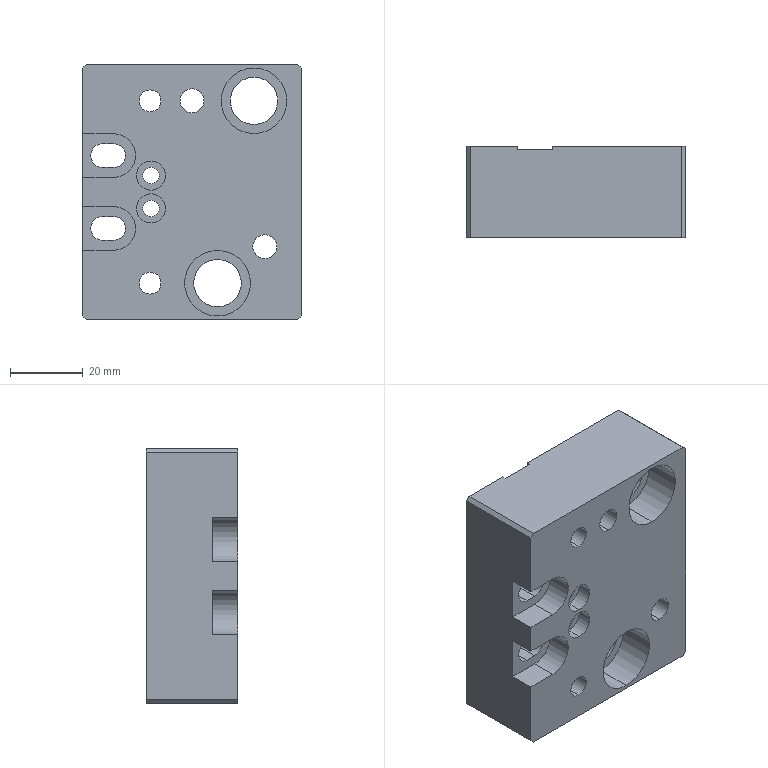Part | SolidWorks | features HoleWzd 7, ICE 3, Chamfer 1, Cut 1, Extrusion 1 | 1 solid | 84 faces | box 60 x 25 x 70 mm | volume 85234 mm3 | cylinder 44 | plane 30 | cone 10 | commonest cylinder face diameters 4.2 x8 4.5 x4 6 x4 6.5 x4 6.6 x4 8 x4